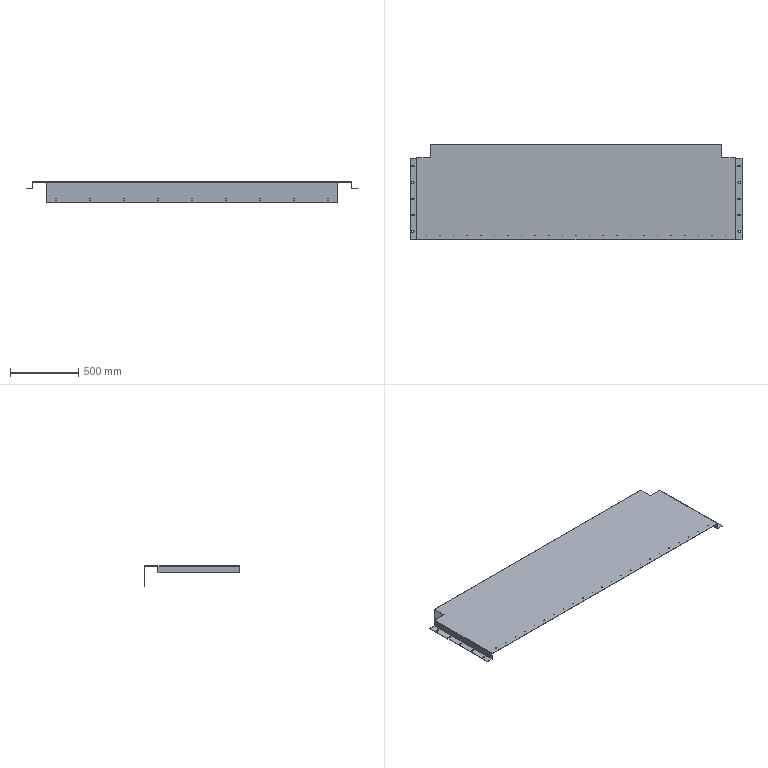Part | SolidWorks | features ICE 4, EdgeFlange 3, LPattern 2, FlatPattern 1, SMBaseFlange 1, SheetMetal 1 | 1 solid | 191 faces | box 2441 x 700 x 150 mm | volume 4096211 mm3 | cylinder 113 | plane 78 | commonest cylinder face diameters 4.5 x46 8.5 x30 6.5 x27 1.473 x5 5.473 x5